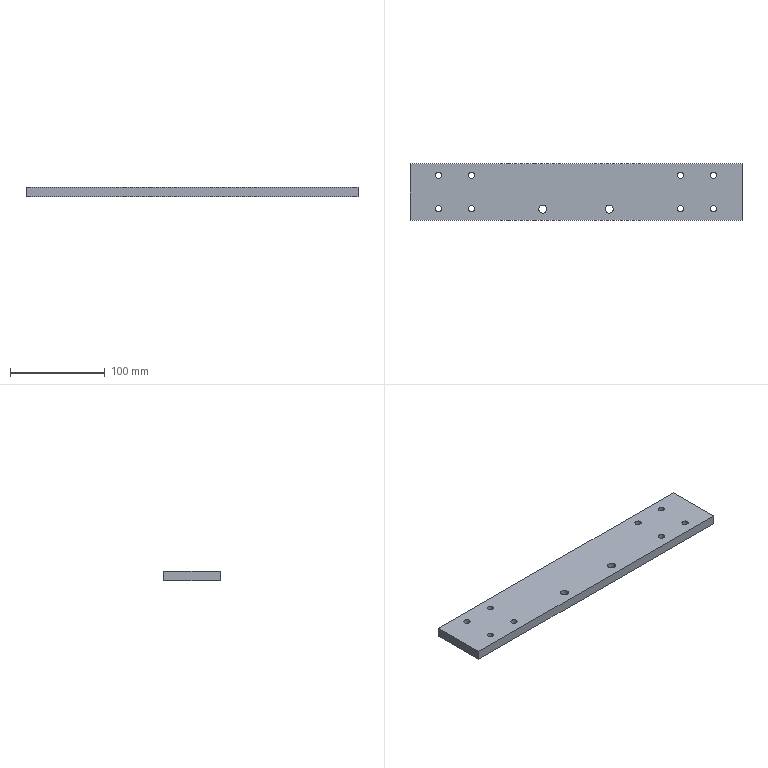Part | SolidWorks | features Extrusion 1, HoleWzd 1 | 1 solid | 26 faces | box 350 x 60 x 10 mm | volume 206210 mm3 | cylinder 20 | plane 6 | commonest cylinder face diameters 6.5 x16 8.5 x4
STEP:
#1=CARTESIAN_POINT('',(-39.25,12.,0.));
#2=VERTEX_POINT('',#1);
#3=CARTESIAN_POINT('',(-30.75,12.,0.));
#4=VERTEX_POINT('',#3);
#5=CARTESIAN_POINT('',(-35.,12.,0.));
#6=DIRECTION('',(0.,0.,1.));
#7=DIRECTION('',(1.,0.,0.));
#8=AXIS2_PLACEMENT_3D('',#5,#6,#7);
#9=CIRCLE('',#8,4.25);
#10=EDGE_CURVE('',#2,#4,#9,.T.);
#11=ORIENTED_EDGE('',*,*,#10,.F.);
#12=CARTESIAN_POINT('',(-39.25,12.,10.));
#13=VERTEX_POINT('',#12);
#14=CARTESIAN_POINT('',(-39.25,12.,10.));
#15=DIRECTION('',(0.,0.,1.));
#16=VECTOR('',#15,1000.);
#17=LINE('',#14,#16);
#18=EDGE_CURVE('',#2,#13,#17,.T.);
#19=ORIENTED_EDGE('',*,*,#18,.T.);
#20=CARTESIAN_POINT('',(-30.75,12.,10.));
#21=VERTEX_POINT('',#20);
#22=CARTESIAN_POINT('',(-35.,12.,10.));
#23=DIRECTION('',(0.,0.,1.));
#24=DIRECTION('',(1.,0.,0.));
#25=AXIS2_PLACEMENT_3D('',#22,#23,#24);
#26=CIRCLE('',#25,4.25);
#27=EDGE_CURVE('',#13,#21,#26,.T.);
#28=ORIENTED_EDGE('',*,*,#27,.T.);
#29=CARTESIAN_POINT('',(-30.75,12.,10.));
#30=DIRECTION('',(0.,0.,1.));
#31=VECTOR('',#30,1000.);
#32=LINE('',#29,#31);
#33=EDGE_CURVE('',#4,#21,#32,.T.);
#34=ORIENTED_EDGE('',*,*,#33,.F.);
#35=EDGE_LOOP('',(#11,#19,#28,#34));
#36=FACE_OUTER_BOUND('',#35,.T.);
#37=CARTESIAN_POINT('',(-35.,12.,10.));
#38=DIRECTION('',(0.,0.,1.));
#39=DIRECTION('',(1.,0.,0.));
#40=AXIS2_PLACEMENT_3D('',#37,#38,#39);
#41=CYLINDRICAL_SURFACE('',#40,4.25);
#42=ADVANCED_FACE('',(#36),#41,.F.);
#43=CARTESIAN_POINT('',(30.75,12.,0.));
#44=VERTEX_POINT('',#43);
#45=CARTESIAN_POINT('',(39.25,12.,0.));
#46=VERTEX_POINT('',#45);
#47=CARTESIAN_POINT('',(35.,12.,0.));
#48=DIRECTION('',(0.,0.,1.));
#49=DIRECTION('',(1.,0.,0.));
#50=AXIS2_PLACEMENT_3D('',#47,#48,#49);
#51=CIRCLE('',#50,4.25);
#52=EDGE_CURVE('',#44,#46,#51,.T.);
#53=ORIENTED_EDGE('',*,*,#52,.F.);
#54=CARTESIAN_POINT('',(30.75,12.,10.));
#55=VERTEX_POINT('',#54);
#56=CARTESIAN_POINT('',(30.75,12.,10.));
#57=DIRECTION('',(0.,0.,1.));
#58=VECTOR('',#57,1000.);
#59=LINE('',#56,#58);
#60=EDGE_CURVE('',#44,#55,#59,.T.);
#61=ORIENTED_EDGE('',*,*,#60,.T.);
#62=CARTESIAN_POINT('',(39.25,12.,10.));
#63=VERTEX_POINT('',#62);
#64=CARTESIAN_POINT('',(35.,12.,10.));
#65=DIRECTION('',(0.,0.,1.));
#66=DIRECTION('',(1.,0.,0.));
#67=AXIS2_PLACEMENT_3D('',#64,#65,#66);
#68=CIRCLE('',#67,4.25);
#69=EDGE_CURVE('',#55,#63,#68,.T.);
#70=ORIENTED_EDGE('',*,*,#69,.T.);
#71=CARTESIAN_POINT('',(39.25,12.,10.));
#72=DIRECTION('',(0.,0.,1.));
#73=VECTOR('',#72,1000.);
#74=LINE('',#71,#73);
#75=EDGE_CURVE('',#46,#63,#74,.T.);
#76=ORIENTED_EDGE('',*,*,#75,.F.);
#77=EDGE_LOOP('',(#53,#61,#70,#76));
#78=FACE_OUTER_BOUND('',#77,.T.);
#79=CARTESIAN_POINT('',(35.,12.,10.));
#80=DIRECTION('',(0.,0.,1.));
#81=DIRECTION('',(1.,0.,0.));
#82=AXIS2_PLACEMENT_3D('',#79,#80,#81);
#83=CYLINDRICAL_SURFACE('',#82,4.25);
#84=ADVANCED_FACE('',(#78),#83,.F.);
#85=CARTESIAN_POINT('',(141.75,47.5,10.));
#86=VERTEX_POINT('',#85);
#87=CARTESIAN_POINT('',(148.25,47.5,10.));
#88=VERTEX_POINT('',#87);
#89=CARTESIAN_POINT('',(145.,47.5,10.));
#90=DIRECTION('',(0.,0.,1.));
#91=DIRECTION('',(-1.,0.,0.));
#92=AXIS2_PLACEMENT_3D('',#89,#90,#91);
#93=CIRCLE('',#92,3.25);
#94=EDGE_CURVE('',#86,#88,#93,.T.);
#95=ORIENTED_EDGE('',*,*,#94,.T.);
#96=CARTESIAN_POINT('',(148.25,47.5,0.));
#97=VERTEX_POINT('',#96);
#98=CARTESIAN_POINT('',(148.25,47.5,10.));
#99=DIRECTION('',(0.,0.,-1.));
#100=VECTOR('',#99,1000.);
#101=LINE('',#98,#100);
#102=EDGE_CURVE('',#88,#97,#101,.T.);
#103=ORIENTED_EDGE('',*,*,#102,.T.);
#104=CARTESIAN_POINT('',(141.75,47.5,0.));
#105=VERTEX_POINT('',#104);
#106=CARTESIAN_POINT('',(145.,47.5,0.));
#107=DIRECTION('',(0.,0.,1.));
#108=DIRECTION('',(-1.,0.,0.));
#109=AXIS2_PLACEMENT_3D('',#106,#107,#108);
#110=CIRCLE('',#109,3.25);
#111=EDGE_CURVE('',#105,#97,#110,.T.);
#112=ORIENTED_EDGE('',*,*,#111,.F.);
#113=CARTESIAN_POINT('',(141.75,47.5,10.));
#114=DIRECTION('',(0.,0.,-1.));
#115=VECTOR('',#114,1000.);
#116=LINE('',#113,#115);
#117=EDGE_CURVE('',#86,#105,#116,.T.);
#118=ORIENTED_EDGE('',*,*,#117,.F.);
#119=EDGE_LOOP('',(#95,#103,#112,#118));
#120=FACE_OUTER_BOUND('',#119,.T.);
#121=CARTESIAN_POINT('',(145.,47.5,10.));
#122=DIRECTION('',(0.,0.,-1.));
#123=DIRECTION('',(-1.,0.,0.));
#124=AXIS2_PLACEMENT_3D('',#121,#122,#123);
#125=CYLINDRICAL_SURFACE('',#124,3.25);
#126=ADVANCED_FACE('',(#120),#125,.F.);
#127=CARTESIAN_POINT('',(106.75,47.5,10.));
#128=VERTEX_POINT('',#127);
#129=CARTESIAN_POINT('',(113.25,47.5,10.));
#130=VERTEX_POINT('',#129);
#131=CARTESIAN_POINT('',(110.,47.5,10.));
#132=DIRECTION('',(0.,0.,1.));
#133=DIRECTION('',(-1.,0.,0.));
#134=AXIS2_PLACEMENT_3D('',#131,#132,#133);
#135=CIRCLE('',#134,3.25);
#136=EDGE_CURVE('',#128,#130,#135,.T.);
#137=ORIENTED_EDGE('',*,*,#136,.T.);
#138=CARTESIAN_POINT('',(113.25,47.5,0.));
#139=VERTEX_POINT('',#138);
#140=CARTESIAN_POINT('',(113.25,47.5,10.));
#141=DIRECTION('',(0.,0.,-1.));
#142=VECTOR('',#141,1000.);
#143=LINE('',#140,#142);
#144=EDGE_CURVE('',#130,#139,#143,.T.);
#145=ORIENTED_EDGE('',*,*,#144,.T.);
#146=CARTESIAN_POINT('',(106.75,47.5,0.));
#147=VERTEX_POINT('',#146);
#148=CARTESIAN_POINT('',(110.,47.5,0.));
#149=DIRECTION('',(0.,0.,1.));
#150=DIRECTION('',(-1.,0.,0.));
#151=AXIS2_PLACEMENT_3D('',#148,#149,#150);
#152=CIRCLE('',#151,3.25);
#153=EDGE_CURVE('',#147,#139,#152,.T.);
#154=ORIENTED_EDGE('',*,*,#153,.F.);
#155=CARTESIAN_POINT('',(106.75,47.5,10.));
#156=DIRECTION('',(0.,0.,-1.));
#157=VECTOR('',#156,1000.);
#158=LINE('',#155,#157);
#159=EDGE_CURVE('',#128,#147,#158,.T.);
#160=ORIENTED_EDGE('',*,*,#159,.F.);
#161=EDGE_LOOP('',(#137,#145,#154,#160));
#162=FACE_OUTER_BOUND('',#161,.T.);
#163=CARTESIAN_POINT('',(110.,47.5,10.));
#164=DIRECTION('',(0.,0.,-1.));
#165=DIRECTION('',(-1.,0.,0.));
#166=AXIS2_PLACEMENT_3D('',#163,#164,#165);
#167=CYLINDRICAL_SURFACE('',#166,3.25);
#168=ADVANCED_FACE('',(#162),#167,.F.);
#169=CARTESIAN_POINT('',(141.75,12.5,10.));
#170=VERTEX_POINT('',#169);
#171=CARTESIAN_POINT('',(148.25,12.5,10.));
#172=VERTEX_POINT('',#171);
#173=CARTESIAN_POINT('',(145.,12.5,10.));
#174=DIRECTION('',(0.,0.,1.));
#175=DIRECTION('',(1.,0.,0.));
#176=AXIS2_PLACEMENT_3D('',#173,#174,#175);
#177=CIRCLE('',#176,3.25);
#178=EDGE_CURVE('',#170,#172,#177,.T.);
#179=ORIENTED_EDGE('',*,*,#178,.T.);
#180=CARTESIAN_POINT('',(148.25,12.5,0.));
#181=VERTEX_POINT('',#180);
#182=CARTESIAN_POINT('',(148.25,12.5,10.));
#183=DIRECTION('',(0.,0.,-1.));
#184=VECTOR('',#183,1000.);
#185=LINE('',#182,#184);
#186=EDGE_CURVE('',#172,#181,#185,.T.);
#187=ORIENTED_EDGE('',*,*,#186,.T.);
#188=CARTESIAN_POINT('',(141.75,12.5,0.));
#189=VERTEX_POINT('',#188);
#190=CARTESIAN_POINT('',(145.,12.5,0.));
#191=DIRECTION('',(0.,0.,1.));
#192=DIRECTION('',(1.,0.,0.));
#193=AXIS2_PLACEMENT_3D('',#190,#191,#192);
#194=CIRCLE('',#193,3.25);
#195=EDGE_CURVE('',#189,#181,#194,.T.);
#196=ORIENTED_EDGE('',*,*,#195,.F.);
#197=CARTESIAN_POINT('',(141.75,12.5,10.));
#198=DIRECTION('',(0.,0.,-1.));
#199=VECTOR('',#198,1000.);
#200=LINE('',#197,#199);
#201=EDGE_CURVE('',#170,#189,#200,.T.);
#202=ORIENTED_EDGE('',*,*,#201,.F.);
#203=EDGE_LOOP('',(#179,#187,#196,#202));
#204=FACE_OUTER_BOUND('',#203,.T.);
#205=CARTESIAN_POINT('',(145.,12.5,10.));
#206=DIRECTION('',(0.,0.,-1.));
#207=DIRECTION('',(-1.,0.,0.));
#208=AXIS2_PLACEMENT_3D('',#205,#206,#207);
#209=CYLINDRICAL_SURFACE('',#208,3.25);
#210=ADVANCED_FACE('',(#204),#209,.F.);
#211=CARTESIAN_POINT('',(106.75,12.5,10.));
#212=VERTEX_POINT('',#211);
#213=CARTESIAN_POINT('',(113.25,12.5,10.));
#214=VERTEX_POINT('',#213);
#215=CARTESIAN_POINT('',(110.,12.5,10.));
#216=DIRECTION('',(0.,0.,1.));
#217=DIRECTION('',(1.,0.,0.));
#218=AXIS2_PLACEMENT_3D('',#215,#216,#217);
#219=CIRCLE('',#218,3.25);
#220=EDGE_CURVE('',#212,#214,#219,.T.);
#221=ORIENTED_EDGE('',*,*,#220,.T.);
#222=CARTESIAN_POINT('',(113.25,12.5,0.));
#223=VERTEX_POINT('',#222);
#224=CARTESIAN_POINT('',(113.25,12.5,10.));
#225=DIRECTION('',(0.,0.,-1.));
#226=VECTOR('',#225,1000.);
#227=LINE('',#224,#226);
#228=EDGE_CURVE('',#214,#223,#227,.T.);
#229=ORIENTED_EDGE('',*,*,#228,.T.);
#230=CARTESIAN_POINT('',(106.75,12.5,0.));
#231=VERTEX_POINT('',#230);
#232=CARTESIAN_POINT('',(110.,12.5,0.));
#233=DIRECTION('',(0.,0.,1.));
#234=DIRECTION('',(1.,0.,0.));
#235=AXIS2_PLACEMENT_3D('',#232,#233,#234);
#236=CIRCLE('',#235,3.25);
#237=EDGE_CURVE('',#231,#223,#236,.T.);
#238=ORIENTED_EDGE('',*,*,#237,.F.);
#239=CARTESIAN_POINT('',(106.75,12.5,10.));
#240=DIRECTION('',(0.,0.,-1.));
#241=VECTOR('',#240,1000.);
#242=LINE('',#239,#241);
#243=EDGE_CURVE('',#212,#231,#242,.T.);
#244=ORIENTED_EDGE('',*,*,#243,.F.);
#245=EDGE_LOOP('',(#221,#229,#238,#244));
#246=FACE_OUTER_BOUND('',#245,.T.);
#247=CARTESIAN_POINT('',(110.,12.5,10.));
#248=DIRECTION('',(0.,0.,-1.));
#249=DIRECTION('',(-1.,0.,0.));
#250=AXIS2_PLACEMENT_3D('',#247,#248,#249);
#251=CYLINDRICAL_SURFACE('',#250,3.25);
#252=ADVANCED_FACE('',(#246),#251,.F.);
#253=CARTESIAN_POINT('',(-148.25,12.5,10.));
#254=VERTEX_POINT('',#253);
#255=CARTESIAN_POINT('',(-141.75,12.5,10.));
#256=VERTEX_POINT('',#255);
#257=CARTESIAN_POINT('',(-145.,12.5,10.));
#258=DIRECTION('',(0.,0.,1.));
#259=DIRECTION('',(-1.,0.,0.));
#260=AXIS2_PLACEMENT_3D('',#257,#258,#259);
#261=CIRCLE('',#260,3.25);
#262=EDGE_CURVE('',#254,#256,#261,.T.);
#263=ORIENTED_EDGE('',*,*,#262,.T.);
#264=CARTESIAN_POINT('',(-141.75,12.5,0.));
#265=VERTEX_POINT('',#264);
#266=CARTESIAN_POINT('',(-141.75,12.5,10.));
#267=DIRECTION('',(0.,0.,-1.));
#268=VECTOR('',#267,1000.);
#269=LINE('',#266,#268);
#270=EDGE_CURVE('',#256,#265,#269,.T.);
#271=ORIENTED_EDGE('',*,*,#270,.T.);
#272=CARTESIAN_POINT('',(-148.25,12.5,0.));
#273=VERTEX_POINT('',#272);
#274=CARTESIAN_POINT('',(-145.,12.5,0.));
#275=DIRECTION('',(0.,0.,1.));
#276=DIRECTION('',(-1.,0.,0.));
#277=AXIS2_PLACEMENT_3D('',#274,#275,#276);
#278=CIRCLE('',#277,3.25);
#279=EDGE_CURVE('',#273,#265,#278,.T.);
#280=ORIENTED_EDGE('',*,*,#279,.F.);
#281=CARTESIAN_POINT('',(-148.25,12.5,10.));
#282=DIRECTION('',(0.,0.,-1.));
#283=VECTOR('',#282,1000.);
#284=LINE('',#281,#283);
#285=EDGE_CURVE('',#254,#273,#284,.T.);
#286=ORIENTED_EDGE('',*,*,#285,.F.);
#287=EDGE_LOOP('',(#263,#271,#280,#286));
#288=FACE_OUTER_BOUND('',#287,.T.);
#289=CARTESIAN_POINT('',(-145.,12.5,10.));
#290=DIRECTION('',(0.,0.,-1.));
#291=DIRECTION('',(-1.,0.,0.));
#292=AXIS2_PLACEMENT_3D('',#289,#290,#291);
#293=CYLINDRICAL_SURFACE('',#292,3.25);
#294=ADVANCED_FACE('',(#288),#293,.F.);
#295=CARTESIAN_POINT('',(-113.25,12.5,10.));
#296=VERTEX_POINT('',#295);
#297=CARTESIAN_POINT('',(-106.75,12.5,10.));
#298=VERTEX_POINT('',#297);
#299=CARTESIAN_POINT('',(-110.,12.5,10.));
#300=DIRECTION('',(0.,0.,1.));
#301=DIRECTION('',(-1.,0.,0.));
#302=AXIS2_PLACEMENT_3D('',#299,#300,#301);
#303=CIRCLE('',#302,3.25);
#304=EDGE_CURVE('',#296,#298,#303,.T.);
#305=ORIENTED_EDGE('',*,*,#304,.T.);
#306=CARTESIAN_POINT('',(-106.75,12.5,0.));
#307=VERTEX_POINT('',#306);
#308=CARTESIAN_POINT('',(-106.75,12.5,10.));
#309=DIRECTION('',(0.,0.,-1.));
#310=VECTOR('',#309,1000.);
#311=LINE('',#308,#310);
#312=EDGE_CURVE('',#298,#307,#311,.T.);
#313=ORIENTED_EDGE('',*,*,#312,.T.);
#314=CARTESIAN_POINT('',(-113.25,12.5,0.));
#315=VERTEX_POINT('',#314);
#316=CARTESIAN_POINT('',(-110.,12.5,0.));
#317=DIRECTION('',(0.,0.,1.));
#318=DIRECTION('',(-1.,0.,0.));
#319=AXIS2_PLACEMENT_3D('',#316,#317,#318);
#320=CIRCLE('',#319,3.25);
#321=EDGE_CURVE('',#315,#307,#320,.T.);
#322=ORIENTED_EDGE('',*,*,#321,.F.);
#323=CARTESIAN_POINT('',(-113.25,12.5,10.));
#324=DIRECTION('',(0.,0.,-1.));
#325=VECTOR('',#324,1000.);
#326=LINE('',#323,#325);
#327=EDGE_CURVE('',#296,#315,#326,.T.);
#328=ORIENTED_EDGE('',*,*,#327,.F.);
#329=EDGE_LOOP('',(#305,#313,#322,#328));
#330=FACE_OUTER_BOUND('',#329,.T.);
#331=CARTESIAN_POINT('',(-110.,12.5,10.));
#332=DIRECTION('',(0.,0.,-1.));
#333=DIRECTION('',(-1.,0.,0.));
#334=AXIS2_PLACEMENT_3D('',#331,#332,#333);
#335=CYLINDRICAL_SURFACE('',#334,3.25);
#336=ADVANCED_FACE('',(#330),#335,.F.);
#337=CARTESIAN_POINT('',(-113.25,47.5,10.));
#338=VERTEX_POINT('',#337);
#339=CARTESIAN_POINT('',(-106.75,47.5,10.));
#340=VERTEX_POINT('',#339);
#341=CARTESIAN_POINT('',(-110.,47.5,10.));
#342=DIRECTION('',(0.,0.,1.));
#343=DIRECTION('',(1.,0.,0.));
#344=AXIS2_PLACEMENT_3D('',#341,#342,#343);
#345=CIRCLE('',#344,3.25);
#346=EDGE_CURVE('',#338,#340,#345,.T.);
#347=ORIENTED_EDGE('',*,*,#346,.T.);
#348=CARTESIAN_POINT('',(-106.75,47.5,0.));
#349=VERTEX_POINT('',#348);
#350=CARTESIAN_POINT('',(-106.75,47.5,10.));
#351=DIRECTION('',(0.,0.,-1.));
#352=VECTOR('',#351,1000.);
#353=LINE('',#350,#352);
#354=EDGE_CURVE('',#340,#349,#353,.T.);
#355=ORIENTED_EDGE('',*,*,#354,.T.);
#356=CARTESIAN_POINT('',(-113.25,47.5,0.));
#357=VERTEX_POINT('',#356);
#358=CARTESIAN_POINT('',(-110.,47.5,0.));
#359=DIRECTION('',(0.,0.,1.));
#360=DIRECTION('',(1.,0.,0.));
#361=AXIS2_PLACEMENT_3D('',#358,#359,#360);
#362=CIRCLE('',#361,3.25);
#363=EDGE_CURVE('',#357,#349,#362,.T.);
#364=ORIENTED_EDGE('',*,*,#363,.F.);
#365=CARTESIAN_POINT('',(-113.25,47.5,10.));
#366=DIRECTION('',(0.,0.,-1.));
#367=VECTOR('',#366,1000.);
#368=LINE('',#365,#367);
#369=EDGE_CURVE('',#338,#357,#368,.T.);
#370=ORIENTED_EDGE('',*,*,#369,.F.);
#371=EDGE_LOOP('',(#347,#355,#364,#370));
#372=FACE_OUTER_BOUND('',#371,.T.);
#373=CARTESIAN_POINT('',(-110.,47.5,10.));
#374=DIRECTION('',(0.,0.,-1.));
#375=DIRECTION('',(-1.,0.,0.));
#376=AXIS2_PLACEMENT_3D('',#373,#374,#375);
#377=CYLINDRICAL_SURFACE('',#376,3.25);
#378=ADVANCED_FACE('',(#372),#377,.F.);
#379=CARTESIAN_POINT('',(-148.25,47.5,10.));
#380=VERTEX_POINT('',#379);
#381=CARTESIAN_POINT('',(-141.75,47.5,10.));
#382=VERTEX_POINT('',#381);
#383=CARTESIAN_POINT('',(-145.,47.5,10.));
#384=DIRECTION('',(0.,0.,1.));
#385=DIRECTION('',(1.,0.,0.));
#386=AXIS2_PLACEMENT_3D('',#383,#384,#385);
#387=CIRCLE('',#386,3.25);
#388=EDGE_CURVE('',#380,#382,#387,.T.);
#389=ORIENTED_EDGE('',*,*,#388,.T.);
#390=CARTESIAN_POINT('',(-141.75,47.5,0.));
#391=VERTEX_POINT('',#390);
#392=CARTESIAN_POINT('',(-141.75,47.5,10.));
#393=DIRECTION('',(0.,0.,-1.));
#394=VECTOR('',#393,1000.);
#395=LINE('',#392,#394);
#396=EDGE_CURVE('',#382,#391,#395,.T.);
#397=ORIENTED_EDGE('',*,*,#396,.T.);
#398=CARTESIAN_POINT('',(-148.25,47.5,0.));
#399=VERTEX_POINT('',#398);
#400=CARTESIAN_POINT('',(-145.,47.5,0.));
#401=DIRECTION('',(0.,0.,1.));
#402=DIRECTION('',(1.,0.,0.));
#403=AXIS2_PLACEMENT_3D('',#400,#401,#402);
#404=CIRCLE('',#403,3.25);
#405=EDGE_CURVE('',#399,#391,#404,.T.);
#406=ORIENTED_EDGE('',*,*,#405,.F.);
#407=CARTESIAN_POINT('',(-148.25,47.5,10.));
#408=DIRECTION('',(0.,0.,-1.));
#409=VECTOR('',#408,1000.);
#410=LINE('',#407,#409);
#411=EDGE_CURVE('',#380,#399,#410,.T.);
#412=ORIENTED_EDGE('',*,*,#411,.F.);
#413=EDGE_LOOP('',(#389,#397,#406,#412));
#414=FACE_OUTER_BOUND('',#413,.T.);
#415=CARTESIAN_POINT('',(-145.,47.5,10.));
#416=DIRECTION('',(0.,0.,-1.));
#417=DIRECTION('',(-1.,0.,0.));
#418=AXIS2_PLACEMENT_3D('',#415,#416,#417);
#419=CYLINDRICAL_SURFACE('',#418,3.25);
#420=ADVANCED_FACE('',(#414),#419,.F.);
#421=CARTESIAN_POINT('',(-35.,12.,10.));
#422=DIRECTION('',(0.,0.,1.));
#423=DIRECTION('',(1.,0.,0.));
#424=AXIS2_PLACEMENT_3D('',#421,#422,#423);
#425=CIRCLE('',#424,4.25);
#426=EDGE_CURVE('',#21,#13,#425,.T.);
#427=ORIENTED_EDGE('',*,*,#426,.F.);
#428=ORIENTED_EDGE('',*,*,#27,.F.);
#429=EDGE_LOOP('',(#427,#428));
#430=FACE_BOUND('',#429,.T.);
#431=CARTESIAN_POINT('',(35.,12.,10.));
#432=DIRECTION('',(0.,0.,1.));
#433=DIRECTION('',(1.,0.,0.));
#434=AXIS2_PLACEMENT_3D('',#431,#432,#433);
#435=CIRCLE('',#434,4.25);
#436=EDGE_CURVE('',#63,#55,#435,.T.);
#437=ORIENTED_EDGE('',*,*,#436,.F.);
#438=ORIENTED_EDGE('',*,*,#69,.F.);
#439=EDGE_LOOP('',(#437,#438));
#440=FACE_BOUND('',#439,.T.);
#441=ORIENTED_EDGE('',*,*,#136,.F.);
#442=CARTESIAN_POINT('',(110.,47.5,10.));
#443=DIRECTION('',(0.,0.,1.));
#444=DIRECTION('',(-1.,0.,0.));
#445=AXIS2_PLACEMENT_3D('',#442,#443,#444);
#446=CIRCLE('',#445,3.25);
#447=EDGE_CURVE('',#130,#128,#446,.T.);
#448=ORIENTED_EDGE('',*,*,#447,.F.);
#449=EDGE_LOOP('',(#441,#448));
#450=FACE_BOUND('',#449,.T.);
#451=ORIENTED_EDGE('',*,*,#220,.F.);
#452=CARTESIAN_POINT('',(110.,12.5,10.));
#453=DIRECTION('',(0.,0.,1.));
#454=DIRECTION('',(1.,0.,0.));
#455=AXIS2_PLACEMENT_3D('',#452,#453,#454);
#456=CIRCLE('',#455,3.25);
#457=EDGE_CURVE('',#214,#212,#456,.T.);
#458=ORIENTED_EDGE('',*,*,#457,.F.);
#459=EDGE_LOOP('',(#451,#458));
#460=FACE_BOUND('',#459,.T.);
#461=ORIENTED_EDGE('',*,*,#304,.F.);
#462=CARTESIAN_POINT('',(-110.,12.5,10.));
#463=DIRECTION('',(0.,0.,1.));
#464=DIRECTION('',(-1.,0.,0.));
#465=AXIS2_PLACEMENT_3D('',#462,#463,#464);
#466=CIRCLE('',#465,3.25);
#467=EDGE_CURVE('',#298,#296,#466,.T.);
#468=ORIENTED_EDGE('',*,*,#467,.F.);
#469=EDGE_LOOP('',(#461,#468));
#470=FACE_BOUND('',#469,.T.);
#471=ORIENTED_EDGE('',*,*,#388,.F.);
#472=CARTESIAN_POINT('',(-145.,47.5,10.));
#473=DIRECTION('',(0.,0.,1.));
#474=DIRECTION('',(1.,0.,0.));
#475=AXIS2_PLACEMENT_3D('',#472,#473,#474);
#476=CIRCLE('',#475,3.25);
#477=EDGE_CURVE('',#382,#380,#476,.T.);
#478=ORIENTED_EDGE('',*,*,#477,.F.);
#479=EDGE_LOOP('',(#471,#478));
#480=FACE_BOUND('',#479,.T.);
#481=CARTESIAN_POINT('',(175.,0.,10.));
#482=VERTEX_POINT('',#481);
#483=CARTESIAN_POINT('',(175.,60.,10.));
#484=VERTEX_POINT('',#483);
#485=CARTESIAN_POINT('',(175.,0.,10.));
#486=DIRECTION('',(0.,1.,0.));
#487=VECTOR('',#486,1000.);
#488=LINE('',#485,#487);
#489=EDGE_CURVE('',#482,#484,#488,.T.);
#490=ORIENTED_EDGE('',*,*,#489,.T.);
#491=CARTESIAN_POINT('',(-175.,60.,10.));
#492=VERTEX_POINT('',#491);
#493=CARTESIAN_POINT('',(175.,60.,10.));
#494=DIRECTION('',(-1.,0.,0.));
#495=VECTOR('',#494,1000.);
#496=LINE('',#493,#495);
#497=EDGE_CURVE('',#484,#492,#496,.T.);
#498=ORIENTED_EDGE('',*,*,#497,.T.);
#499=CARTESIAN_POINT('',(-175.,0.,10.));
#500=VERTEX_POINT('',#499);
#501=CARTESIAN_POINT('',(-175.,0.,10.));
#502=DIRECTION('',(0.,-1.,0.));
#503=VECTOR('',#502,1000.);
#504=LINE('',#501,#503);
#505=EDGE_CURVE('',#492,#500,#504,.T.);
#506=ORIENTED_EDGE('',*,*,#505,.T.);
#507=CARTESIAN_POINT('',(175.,0.,10.));
#508=DIRECTION('',(1.,0.,0.));
#509=VECTOR('',#508,1000.);
#510=LINE('',#507,#509);
#511=EDGE_CURVE('',#500,#482,#510,.T.);
#512=ORIENTED_EDGE('',*,*,#511,.T.);
#513=EDGE_LOOP('',(#490,#498,#506,#512));
#514=FACE_OUTER_BOUND('',#513,.T.);
#515=ORIENTED_EDGE('',*,*,#346,.F.);
#516=CARTESIAN_POINT('',(-110.,47.5,10.));
#517=DIRECTION('',(0.,0.,1.));
#518=DIRECTION('',(1.,0.,0.));
#519=AXIS2_PLACEMENT_3D('',#516,#517,#518);
#520=CIRCLE('',#519,3.25);
#521=EDGE_CURVE('',#340,#338,#520,.T.);
#522=ORIENTED_EDGE('',*,*,#521,.F.);
#523=EDGE_LOOP('',(#515,#522));
#524=FACE_BOUND('',#523,.T.);
#525=ORIENTED_EDGE('',*,*,#262,.F.);
#526=CARTESIAN_POINT('',(-145.,12.5,10.));
#527=DIRECTION('',(0.,0.,1.));
#528=DIRECTION('',(-1.,0.,0.));
#529=AXIS2_PLACEMENT_3D('',#526,#527,#528);
#530=CIRCLE('',#529,3.25);
#531=EDGE_CURVE('',#256,#254,#530,.T.);
#532=ORIENTED_EDGE('',*,*,#531,.F.);
#533=EDGE_LOOP('',(#525,#532));
#534=FACE_BOUND('',#533,.T.);
#535=ORIENTED_EDGE('',*,*,#178,.F.);
#536=CARTESIAN_POINT('',(145.,12.5,10.));
#537=DIRECTION('',(0.,0.,1.));
#538=DIRECTION('',(1.,0.,0.));
#539=AXIS2_PLACEMENT_3D('',#536,#537,#538);
#540=CIRCLE('',#539,3.25);
#541=EDGE_CURVE('',#172,#170,#540,.T.);
#542=ORIENTED_EDGE('',*,*,#541,.F.);
#543=EDGE_LOOP('',(#535,#542));
#544=FACE_BOUND('',#543,.T.);
#545=ORIENTED_EDGE('',*,*,#94,.F.);
#546=CARTESIAN_POINT('',(145.,47.5,10.));
#547=DIRECTION('',(0.,0.,1.));
#548=DIRECTION('',(-1.,0.,0.));
#549=AXIS2_PLACEMENT_3D('',#546,#547,#548);
#550=CIRCLE('',#549,3.25);
#551=EDGE_CURVE('',#88,#86,#550,.T.);
#552=ORIENTED_EDGE('',*,*,#551,.F.);
#553=EDGE_LOOP('',(#545,#552));
#554=FACE_BOUND('',#553,.T.);
#555=CARTESIAN_POINT('',(0.,0.,10.));
#556=DIRECTION('',(0.,0.,1.));
#557=DIRECTION('',(1.,0.,0.));
#558=AXIS2_PLACEMENT_3D('',#555,#556,#557);
#559=PLANE('',#558);
#560=ADVANCED_FACE('',(#430,#440,#450,#460,#470,#480,#514,#524,#534,#544,#554),#559,.T.);
#561=CARTESIAN_POINT('',(-35.,12.,0.));
#562=DIRECTION('',(0.,0.,1.));
#563=DIRECTION('',(1.,0.,0.));
#564=AXIS2_PLACEMENT_3D('',#561,#562,#563);
#565=CIRCLE('',#564,4.25);
#566=EDGE_CURVE('',#4,#2,#565,.T.);
#567=ORIENTED_EDGE('',*,*,#566,.T.);
#568=ORIENTED_EDGE('',*,*,#10,.T.);
#569=EDGE_LOOP('',(#567,#568));
#570=FACE_BOUND('',#569,.T.);
#571=CARTESIAN_POINT('',(35.,12.,0.));
#572=DIRECTION('',(0.,0.,1.));
#573=DIRECTION('',(1.,0.,0.));
#574=AXIS2_PLACEMENT_3D('',#571,#572,#573);
#575=CIRCLE('',#574,4.25);
#576=EDGE_CURVE('',#46,#44,#575,.T.);
#577=ORIENTED_EDGE('',*,*,#576,.T.);
#578=ORIENTED_EDGE('',*,*,#52,.T.);
#579=EDGE_LOOP('',(#577,#578));
#580=FACE_BOUND('',#579,.T.);
#581=CARTESIAN_POINT('',(175.,0.,0.));
#582=VERTEX_POINT('',#581);
#583=CARTESIAN_POINT('',(175.,60.,0.));
#584=VERTEX_POINT('',#583);
#585=CARTESIAN_POINT('',(175.,0.,0.));
#586=DIRECTION('',(0.,1.,0.));
#587=VECTOR('',#586,1000.);
#588=LINE('',#585,#587);
#589=EDGE_CURVE('',#582,#584,#588,.T.);
#590=ORIENTED_EDGE('',*,*,#589,.F.);
#591=CARTESIAN_POINT('',(-175.,0.,0.));
#592=VERTEX_POINT('',#591);
#593=CARTESIAN_POINT('',(175.,0.,0.));
#594=DIRECTION('',(1.,0.,0.));
#595=VECTOR('',#594,1000.);
#596=LINE('',#593,#595);
#597=EDGE_CURVE('',#592,#582,#596,.T.);
#598=ORIENTED_EDGE('',*,*,#597,.F.);
#599=CARTESIAN_POINT('',(-175.,60.,0.));
#600=VERTEX_POINT('',#599);
#601=CARTESIAN_POINT('',(-175.,0.,0.));
#602=DIRECTION('',(0.,-1.,0.));
#603=VECTOR('',#602,1000.);
#604=LINE('',#601,#603);
#605=EDGE_CURVE('',#600,#592,#604,.T.);
#606=ORIENTED_EDGE('',*,*,#605,.F.);
#607=CARTESIAN_POINT('',(175.,60.,0.));
#608=DIRECTION('',(-1.,0.,0.));
#609=VECTOR('',#608,1000.);
#610=LINE('',#607,#609);
#611=EDGE_CURVE('',#584,#600,#610,.T.);
#612=ORIENTED_EDGE('',*,*,#611,.F.);
#613=EDGE_LOOP('',(#590,#598,#606,#612));
#614=FACE_OUTER_BOUND('',#613,.T.);
#615=ORIENTED_EDGE('',*,*,#405,.T.);
#616=CARTESIAN_POINT('',(-145.,47.5,0.));
#617=DIRECTION('',(0.,0.,1.));
#618=DIRECTION('',(1.,0.,0.));
#619=AXIS2_PLACEMENT_3D('',#616,#617,#618);
#620=CIRCLE('',#619,3.25);
#621=EDGE_CURVE('',#391,#399,#620,.T.);
#622=ORIENTED_EDGE('',*,*,#621,.T.);
#623=EDGE_LOOP('',(#615,#622));
#624=FACE_BOUND('',#623,.T.);
#625=ORIENTED_EDGE('',*,*,#363,.T.);
#626=CARTESIAN_POINT('',(-110.,47.5,0.));
#627=DIRECTION('',(0.,0.,1.));
#628=DIRECTION('',(1.,0.,0.));
#629=AXIS2_PLACEMENT_3D('',#626,#627,#628);
#630=CIRCLE('',#629,3.25);
#631=EDGE_CURVE('',#349,#357,#630,.T.);
#632=ORIENTED_EDGE('',*,*,#631,.T.);
#633=EDGE_LOOP('',(#625,#632));
#634=FACE_BOUND('',#633,.T.);
#635=ORIENTED_EDGE('',*,*,#321,.T.);
#636=CARTESIAN_POINT('',(-110.,12.5,0.));
#637=DIRECTION('',(0.,0.,1.));
#638=DIRECTION('',(-1.,0.,0.));
#639=AXIS2_PLACEMENT_3D('',#636,#637,#638);
#640=CIRCLE('',#639,3.25);
#641=EDGE_CURVE('',#307,#315,#640,.T.);
#642=ORIENTED_EDGE('',*,*,#641,.T.);
#643=EDGE_LOOP('',(#635,#642));
#644=FACE_BOUND('',#643,.T.);
#645=ORIENTED_EDGE('',*,*,#279,.T.);
#646=CARTESIAN_POINT('',(-145.,12.5,0.));
#647=DIRECTION('',(0.,0.,1.));
#648=DIRECTION('',(-1.,0.,0.));
#649=AXIS2_PLACEMENT_3D('',#646,#647,#648);
#650=CIRCLE('',#649,3.25);
#651=EDGE_CURVE('',#265,#273,#650,.T.);
#652=ORIENTED_EDGE('',*,*,#651,.T.);
#653=EDGE_LOOP('',(#645,#652));
#654=FACE_BOUND('',#653,.T.);
#655=ORIENTED_EDGE('',*,*,#237,.T.);
#656=CARTESIAN_POINT('',(110.,12.5,0.));
#657=DIRECTION('',(0.,0.,1.));
#658=DIRECTION('',(1.,0.,0.));
#659=AXIS2_PLACEMENT_3D('',#656,#657,#658);
#660=CIRCLE('',#659,3.25);
#661=EDGE_CURVE('',#223,#231,#660,.T.);
#662=ORIENTED_EDGE('',*,*,#661,.T.);
#663=EDGE_LOOP('',(#655,#662));
#664=FACE_BOUND('',#663,.T.);
#665=ORIENTED_EDGE('',*,*,#195,.T.);
#666=CARTESIAN_POINT('',(145.,12.5,0.));
#667=DIRECTION('',(0.,0.,1.));
#668=DIRECTION('',(1.,0.,0.));
#669=AXIS2_PLACEMENT_3D('',#666,#667,#668);
#670=CIRCLE('',#669,3.25);
#671=EDGE_CURVE('',#181,#189,#670,.T.);
#672=ORIENTED_EDGE('',*,*,#671,.T.);
#673=EDGE_LOOP('',(#665,#672));
#674=FACE_BOUND('',#673,.T.);
#675=ORIENTED_EDGE('',*,*,#153,.T.);
#676=CARTESIAN_POINT('',(110.,47.5,0.));
#677=DIRECTION('',(0.,0.,1.));
#678=DIRECTION('',(-1.,0.,0.));
#679=AXIS2_PLACEMENT_3D('',#676,#677,#678);
#680=CIRCLE('',#679,3.25);
#681=EDGE_CURVE('',#139,#147,#680,.T.);
#682=ORIENTED_EDGE('',*,*,#681,.T.);
#683=EDGE_LOOP('',(#675,#682));
#684=FACE_BOUND('',#683,.T.);
#685=ORIENTED_EDGE('',*,*,#111,.T.);
#686=CARTESIAN_POINT('',(145.,47.5,0.));
#687=DIRECTION('',(0.,0.,1.));
#688=DIRECTION('',(-1.,0.,0.));
#689=AXIS2_PLACEMENT_3D('',#686,#687,#688);
#690=CIRCLE('',#689,3.25);
#691=EDGE_CURVE('',#97,#105,#690,.T.);
#692=ORIENTED_EDGE('',*,*,#691,.T.);
#693=EDGE_LOOP('',(#685,#692));
#694=FACE_BOUND('',#693,.T.);
#695=CARTESIAN_POINT('',(0.,0.,0.));
#696=DIRECTION('',(0.,0.,1.));
#697=DIRECTION('',(1.,0.,0.));
#698=AXIS2_PLACEMENT_3D('',#695,#696,#697);
#699=PLANE('',#698);
#700=ADVANCED_FACE('',(#570,#580,#614,#624,#634,#644,#654,#664,#674,#684,#694),#699,.F.);
#701=ORIENTED_EDGE('',*,*,#589,.T.);
#702=CARTESIAN_POINT('',(175.,60.,10.));
#703=DIRECTION('',(0.,0.,-1.));
#704=VECTOR('',#703,1000.);
#705=LINE('',#702,#704);
#706=EDGE_CURVE('',#484,#584,#705,.T.);
#707=ORIENTED_EDGE('',*,*,#706,.F.);
#708=ORIENTED_EDGE('',*,*,#489,.F.);
#709=CARTESIAN_POINT('',(175.,0.,10.));
#710=DIRECTION('',(0.,0.,-1.));
#711=VECTOR('',#710,1000.);
#712=LINE('',#709,#711);
#713=EDGE_CURVE('',#482,#582,#712,.T.);
#714=ORIENTED_EDGE('',*,*,#713,.T.);
#715=EDGE_LOOP('',(#701,#707,#708,#714));
#716=FACE_OUTER_BOUND('',#715,.T.);
#717=CARTESIAN_POINT('',(175.,0.,10.));
#718=DIRECTION('',(-1.,0.,0.));
#719=DIRECTION('',(0.,0.,1.));
#720=AXIS2_PLACEMENT_3D('',#717,#718,#719);
#721=PLANE('',#720);
#722=ADVANCED_FACE('',(#716),#721,.F.);
#723=ORIENTED_EDGE('',*,*,#611,.T.);
#724=CARTESIAN_POINT('',(-175.,60.,10.));
#725=DIRECTION('',(0.,0.,-1.));
#726=VECTOR('',#725,1000.);
#727=LINE('',#724,#726);
#728=EDGE_CURVE('',#492,#600,#727,.T.);
#729=ORIENTED_EDGE('',*,*,#728,.F.);
#730=ORIENTED_EDGE('',*,*,#497,.F.);
#731=ORIENTED_EDGE('',*,*,#706,.T.);
#732=EDGE_LOOP('',(#723,#729,#730,#731));
#733=FACE_OUTER_BOUND('',#732,.T.);
#734=CARTESIAN_POINT('',(175.,60.,10.));
#735=DIRECTION('',(0.,-1.,0.));
#736=DIRECTION('',(0.,0.,-1.));
#737=AXIS2_PLACEMENT_3D('',#734,#735,#736);
#738=PLANE('',#737);
#739=ADVANCED_FACE('',(#733),#738,.F.);
#740=ORIENTED_EDGE('',*,*,#605,.T.);
#741=CARTESIAN_POINT('',(-175.,0.,10.));
#742=DIRECTION('',(0.,0.,-1.));
#743=VECTOR('',#742,1000.);
#744=LINE('',#741,#743);
#745=EDGE_CURVE('',#500,#592,#744,.T.);
#746=ORIENTED_EDGE('',*,*,#745,.F.);
#747=ORIENTED_EDGE('',*,*,#505,.F.);
#748=ORIENTED_EDGE('',*,*,#728,.T.);
#749=EDGE_LOOP('',(#740,#746,#747,#748));
#750=FACE_OUTER_BOUND('',#749,.T.);
#751=CARTESIAN_POINT('',(-175.,0.,10.));
#752=DIRECTION('',(1.,0.,0.));
#753=DIRECTION('',(0.,0.,-1.));
#754=AXIS2_PLACEMENT_3D('',#751,#752,#753);
#755=PLANE('',#754);
#756=ADVANCED_FACE('',(#750),#755,.F.);
#757=ORIENTED_EDGE('',*,*,#597,.T.);
#758=ORIENTED_EDGE('',*,*,#713,.F.);
#759=ORIENTED_EDGE('',*,*,#511,.F.);
#760=ORIENTED_EDGE('',*,*,#745,.T.);
#761=EDGE_LOOP('',(#757,#758,#759,#760));
#762=FACE_OUTER_BOUND('',#761,.T.);
#763=CARTESIAN_POINT('',(175.,0.,10.));
#764=DIRECTION('',(0.,1.,0.));
#765=DIRECTION('',(-1.,0.,0.));
#766=AXIS2_PLACEMENT_3D('',#763,#764,#765);
#767=PLANE('',#766);
#768=ADVANCED_FACE('',(#762),#767,.F.);
#769=ORIENTED_EDGE('',*,*,#396,.F.);
#770=ORIENTED_EDGE('',*,*,#477,.T.);
#771=ORIENTED_EDGE('',*,*,#411,.T.);
#772=ORIENTED_EDGE('',*,*,#621,.F.);
#773=EDGE_LOOP('',(#769,#770,#771,#772));
#774=FACE_OUTER_BOUND('',#773,.T.);
#775=CARTESIAN_POINT('',(-145.,47.5,10.));
#776=DIRECTION('',(0.,0.,-1.));
#777=DIRECTION('',(-1.,0.,0.));
#778=AXIS2_PLACEMENT_3D('',#775,#776,#777);
#779=CYLINDRICAL_SURFACE('',#778,3.25);
#780=ADVANCED_FACE('',(#774),#779,.F.);
#781=ORIENTED_EDGE('',*,*,#354,.F.);
#782=ORIENTED_EDGE('',*,*,#521,.T.);
#783=ORIENTED_EDGE('',*,*,#369,.T.);
#784=ORIENTED_EDGE('',*,*,#631,.F.);
#785=EDGE_LOOP('',(#781,#782,#783,#784));
#786=FACE_OUTER_BOUND('',#785,.T.);
#787=CARTESIAN_POINT('',(-110.,47.5,10.));
#788=DIRECTION('',(0.,0.,-1.));
#789=DIRECTION('',(-1.,0.,0.));
#790=AXIS2_PLACEMENT_3D('',#787,#788,#789);
#791=CYLINDRICAL_SURFACE('',#790,3.25);
#792=ADVANCED_FACE('',(#786),#791,.F.);
#793=ORIENTED_EDGE('',*,*,#312,.F.);
#794=ORIENTED_EDGE('',*,*,#467,.T.);
#795=ORIENTED_EDGE('',*,*,#327,.T.);
#796=ORIENTED_EDGE('',*,*,#641,.F.);
#797=EDGE_LOOP('',(#793,#794,#795,#796));
#798=FACE_OUTER_BOUND('',#797,.T.);
#799=CARTESIAN_POINT('',(-110.,12.5,10.));
#800=DIRECTION('',(0.,0.,-1.));
#801=DIRECTION('',(-1.,0.,0.));
#802=AXIS2_PLACEMENT_3D('',#799,#800,#801);
#803=CYLINDRICAL_SURFACE('',#802,3.25);
#804=ADVANCED_FACE('',(#798),#803,.F.);
#805=ORIENTED_EDGE('',*,*,#270,.F.);
#806=ORIENTED_EDGE('',*,*,#531,.T.);
#807=ORIENTED_EDGE('',*,*,#285,.T.);
#808=ORIENTED_EDGE('',*,*,#651,.F.);
#809=EDGE_LOOP('',(#805,#806,#807,#808));
#810=FACE_OUTER_BOUND('',#809,.T.);
#811=CARTESIAN_POINT('',(-145.,12.5,10.));
#812=DIRECTION('',(0.,0.,-1.));
#813=DIRECTION('',(-1.,0.,0.));
#814=AXIS2_PLACEMENT_3D('',#811,#812,#813);
#815=CYLINDRICAL_SURFACE('',#814,3.25);
#816=ADVANCED_FACE('',(#810),#815,.F.);
#817=ORIENTED_EDGE('',*,*,#228,.F.);
#818=ORIENTED_EDGE('',*,*,#457,.T.);
#819=ORIENTED_EDGE('',*,*,#243,.T.);
#820=ORIENTED_EDGE('',*,*,#661,.F.);
#821=EDGE_LOOP('',(#817,#818,#819,#820));
#822=FACE_OUTER_BOUND('',#821,.T.);
#823=CARTESIAN_POINT('',(110.,12.5,10.));
#824=DIRECTION('',(0.,0.,-1.));
#825=DIRECTION('',(-1.,0.,0.));
#826=AXIS2_PLACEMENT_3D('',#823,#824,#825);
#827=CYLINDRICAL_SURFACE('',#826,3.25);
#828=ADVANCED_FACE('',(#822),#827,.F.);
#829=ORIENTED_EDGE('',*,*,#186,.F.);
#830=ORIENTED_EDGE('',*,*,#541,.T.);
#831=ORIENTED_EDGE('',*,*,#201,.T.);
#832=ORIENTED_EDGE('',*,*,#671,.F.);
#833=EDGE_LOOP('',(#829,#830,#831,#832));
#834=FACE_OUTER_BOUND('',#833,.T.);
#835=CARTESIAN_POINT('',(145.,12.5,10.));
#836=DIRECTION('',(0.,0.,-1.));
#837=DIRECTION('',(-1.,0.,0.));
#838=AXIS2_PLACEMENT_3D('',#835,#836,#837);
#839=CYLINDRICAL_SURFACE('',#838,3.25);
#840=ADVANCED_FACE('',(#834),#839,.F.);
#841=ORIENTED_EDGE('',*,*,#144,.F.);
#842=ORIENTED_EDGE('',*,*,#447,.T.);
#843=ORIENTED_EDGE('',*,*,#159,.T.);
#844=ORIENTED_EDGE('',*,*,#681,.F.);
#845=EDGE_LOOP('',(#841,#842,#843,#844));
#846=FACE_OUTER_BOUND('',#845,.T.);
#847=CARTESIAN_POINT('',(110.,47.5,10.));
#848=DIRECTION('',(0.,0.,-1.));
#849=DIRECTION('',(-1.,0.,0.));
#850=AXIS2_PLACEMENT_3D('',#847,#848,#849);
#851=CYLINDRICAL_SURFACE('',#850,3.25);
#852=ADVANCED_FACE('',(#846),#851,.F.);
#853=ORIENTED_EDGE('',*,*,#102,.F.);
#854=ORIENTED_EDGE('',*,*,#551,.T.);
#855=ORIENTED_EDGE('',*,*,#117,.T.);
#856=ORIENTED_EDGE('',*,*,#691,.F.);
#857=EDGE_LOOP('',(#853,#854,#855,#856));
#858=FACE_OUTER_BOUND('',#857,.T.);
#859=CARTESIAN_POINT('',(145.,47.5,10.));
#860=DIRECTION('',(0.,0.,-1.));
#861=DIRECTION('',(-1.,0.,0.));
#862=AXIS2_PLACEMENT_3D('',#859,#860,#861);
#863=CYLINDRICAL_SURFACE('',#862,3.25);
#864=ADVANCED_FACE('',(#858),#863,.F.);
#865=ORIENTED_EDGE('',*,*,#60,.F.);
#866=ORIENTED_EDGE('',*,*,#576,.F.);
#867=ORIENTED_EDGE('',*,*,#75,.T.);
#868=ORIENTED_EDGE('',*,*,#436,.T.);
#869=EDGE_LOOP('',(#865,#866,#867,#868));
#870=FACE_OUTER_BOUND('',#869,.T.);
#871=CARTESIAN_POINT('',(35.,12.,10.));
#872=DIRECTION('',(0.,0.,1.));
#873=DIRECTION('',(1.,0.,0.));
#874=AXIS2_PLACEMENT_3D('',#871,#872,#873);
#875=CYLINDRICAL_SURFACE('',#874,4.25);
#876=ADVANCED_FACE('',(#870),#875,.F.);
#877=ORIENTED_EDGE('',*,*,#18,.F.);
#878=ORIENTED_EDGE('',*,*,#566,.F.);
#879=ORIENTED_EDGE('',*,*,#33,.T.);
#880=ORIENTED_EDGE('',*,*,#426,.T.);
#881=EDGE_LOOP('',(#877,#878,#879,#880));
#882=FACE_OUTER_BOUND('',#881,.T.);
#883=CARTESIAN_POINT('',(-35.,12.,10.));
#884=DIRECTION('',(0.,0.,1.));
#885=DIRECTION('',(1.,0.,0.));
#886=AXIS2_PLACEMENT_3D('',#883,#884,#885);
#887=CYLINDRICAL_SURFACE('',#886,4.25);
#888=ADVANCED_FACE('',(#882),#887,.F.);
#889=CLOSED_SHELL('',(#42,#84,#126,#168,#210,#252,#294,#336,#378,#420,#560,#700,#722,#739,#756,#768,#780,#792,#804,#816,#828,#840,#852,#864,#876,#888));
#890=MANIFOLD_SOLID_BREP('',#889);
#891=CARTESIAN_POINT('',(0.,0.,0.));
#892=DIRECTION('',(0.,0.,1.));
#893=DIRECTION('',(1.,0.,0.));
#894=AXIS2_PLACEMENT_3D('',#891,#892,#893);
#895=(LENGTH_UNIT()NAMED_UNIT(*)SI_UNIT(.MILLI.,.METRE.));
#896=UNCERTAINTY_MEASURE_WITH_UNIT(LENGTH_MEASURE(0.00001),#895,'','');
#897=(NAMED_UNIT(*)PLANE_ANGLE_UNIT()SI_UNIT($,.RADIAN.));
#898=(NAMED_UNIT(*)SI_UNIT($,.STERADIAN.)SOLID_ANGLE_UNIT());
#899=(GEOMETRIC_REPRESENTATION_CONTEXT(3)GLOBAL_UNCERTAINTY_ASSIGNED_CONTEXT((#896))GLOBAL_UNIT_ASSIGNED_CONTEXT((#895,#897,#898))REPRESENTATION_CONTEXT('',''));
#900=ADVANCED_BREP_SHAPE_REPRESENTATION('',(#890,#894),#899);